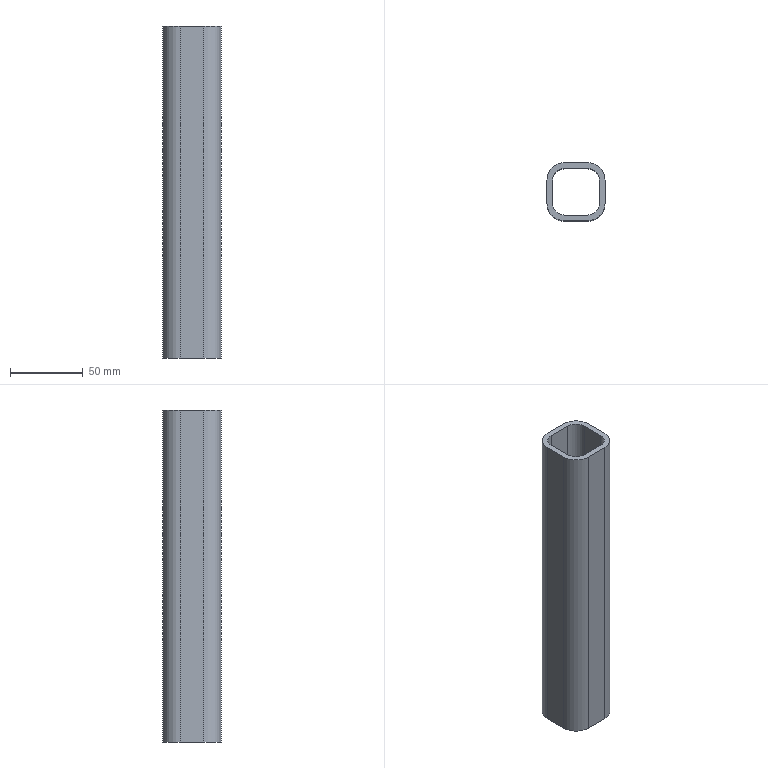Part | SolidWorks | features BaseBody 1 | 1 solid | 18 faces | box 40 x 40 x 228 mm | volume 115671 mm3 | plane 10 | cylinder 8 | commonest cylinder face diameters 16 x4 24 x4
STEP:
#1=CARTESIAN_POINT('',(8.,-20.,0.));
#2=VERTEX_POINT('',#1);
#3=CARTESIAN_POINT('',(20.,-8.,0.));
#4=VERTEX_POINT('',#3);
#5=CARTESIAN_POINT('',(8.,-8.,0.));
#6=DIRECTION('',(0.,0.,1.));
#7=DIRECTION('',(1.,0.,0.));
#8=AXIS2_PLACEMENT_3D('',#5,#6,#7);
#9=CIRCLE('',#8,12.);
#10=EDGE_CURVE('',#2,#4,#9,.T.);
#11=ORIENTED_EDGE('',*,*,#10,.T.);
#12=CARTESIAN_POINT('',(20.,-8.,228.));
#13=VERTEX_POINT('',#12);
#14=CARTESIAN_POINT('',(20.,-8.,0.));
#15=DIRECTION('',(0.,0.,1.));
#16=VECTOR('',#15,1000.);
#17=LINE('',#14,#16);
#18=EDGE_CURVE('',#4,#13,#17,.T.);
#19=ORIENTED_EDGE('',*,*,#18,.T.);
#20=CARTESIAN_POINT('',(8.,-20.,228.));
#21=VERTEX_POINT('',#20);
#22=CARTESIAN_POINT('',(8.,-8.,228.));
#23=DIRECTION('',(0.,0.,-1.));
#24=DIRECTION('',(1.,0.,0.));
#25=AXIS2_PLACEMENT_3D('',#22,#23,#24);
#26=CIRCLE('',#25,12.);
#27=EDGE_CURVE('',#13,#21,#26,.T.);
#28=ORIENTED_EDGE('',*,*,#27,.T.);
#29=CARTESIAN_POINT('',(8.,-20.,0.));
#30=DIRECTION('',(0.,0.,-1.));
#31=VECTOR('',#30,1000.);
#32=LINE('',#29,#31);
#33=EDGE_CURVE('',#21,#2,#32,.T.);
#34=ORIENTED_EDGE('',*,*,#33,.T.);
#35=EDGE_LOOP('',(#11,#19,#28,#34));
#36=FACE_OUTER_BOUND('',#35,.T.);
#37=CARTESIAN_POINT('',(8.,-8.,0.));
#38=DIRECTION('',(0.,0.,1.));
#39=DIRECTION('',(1.,0.,0.));
#40=AXIS2_PLACEMENT_3D('',#37,#38,#39);
#41=CYLINDRICAL_SURFACE('',#40,12.);
#42=ADVANCED_FACE('',(#36),#41,.T.);
#43=CARTESIAN_POINT('',(20.,8.,0.));
#44=VERTEX_POINT('',#43);
#45=CARTESIAN_POINT('',(20.,8.,0.));
#46=DIRECTION('',(0.,1.,0.));
#47=VECTOR('',#46,1000.);
#48=LINE('',#45,#47);
#49=EDGE_CURVE('',#4,#44,#48,.T.);
#50=ORIENTED_EDGE('',*,*,#49,.T.);
#51=CARTESIAN_POINT('',(20.,8.,228.));
#52=VERTEX_POINT('',#51);
#53=CARTESIAN_POINT('',(20.,8.,0.));
#54=DIRECTION('',(0.,0.,1.));
#55=VECTOR('',#54,1000.);
#56=LINE('',#53,#55);
#57=EDGE_CURVE('',#44,#52,#56,.T.);
#58=ORIENTED_EDGE('',*,*,#57,.T.);
#59=CARTESIAN_POINT('',(20.,8.,228.));
#60=DIRECTION('',(0.,-1.,0.));
#61=VECTOR('',#60,1000.);
#62=LINE('',#59,#61);
#63=EDGE_CURVE('',#52,#13,#62,.T.);
#64=ORIENTED_EDGE('',*,*,#63,.T.);
#65=ORIENTED_EDGE('',*,*,#18,.F.);
#66=EDGE_LOOP('',(#50,#58,#64,#65));
#67=FACE_OUTER_BOUND('',#66,.T.);
#68=CARTESIAN_POINT('',(20.,8.,0.));
#69=DIRECTION('',(1.,0.,0.));
#70=DIRECTION('',(0.,1.,0.));
#71=AXIS2_PLACEMENT_3D('',#68,#69,#70);
#72=PLANE('',#71);
#73=ADVANCED_FACE('',(#67),#72,.T.);
#74=CARTESIAN_POINT('',(-16.,8.,0.));
#75=VERTEX_POINT('',#74);
#76=CARTESIAN_POINT('',(-8.,16.,0.));
#77=VERTEX_POINT('',#76);
#78=CARTESIAN_POINT('',(-8.,8.,0.));
#79=DIRECTION('',(0.,0.,-1.));
#80=DIRECTION('',(1.,0.,0.));
#81=AXIS2_PLACEMENT_3D('',#78,#79,#80);
#82=CIRCLE('',#81,8.);
#83=EDGE_CURVE('',#75,#77,#82,.T.);
#84=ORIENTED_EDGE('',*,*,#83,.F.);
#85=CARTESIAN_POINT('',(-16.,-8.,0.));
#86=VERTEX_POINT('',#85);
#87=CARTESIAN_POINT('',(-16.,0.,0.));
#88=DIRECTION('',(0.,1.,0.));
#89=VECTOR('',#88,1000.);
#90=LINE('',#87,#89);
#91=EDGE_CURVE('',#86,#75,#90,.T.);
#92=ORIENTED_EDGE('',*,*,#91,.F.);
#93=CARTESIAN_POINT('',(-8.,-16.,0.));
#94=VERTEX_POINT('',#93);
#95=CARTESIAN_POINT('',(-8.,-8.,0.));
#96=DIRECTION('',(0.,0.,-1.));
#97=DIRECTION('',(1.,0.,0.));
#98=AXIS2_PLACEMENT_3D('',#95,#96,#97);
#99=CIRCLE('',#98,8.);
#100=EDGE_CURVE('',#94,#86,#99,.T.);
#101=ORIENTED_EDGE('',*,*,#100,.F.);
#102=CARTESIAN_POINT('',(8.,-16.,0.));
#103=VERTEX_POINT('',#102);
#104=CARTESIAN_POINT('',(0.,-16.,0.));
#105=DIRECTION('',(-1.,0.,0.));
#106=VECTOR('',#105,1000.);
#107=LINE('',#104,#106);
#108=EDGE_CURVE('',#103,#94,#107,.T.);
#109=ORIENTED_EDGE('',*,*,#108,.F.);
#110=CARTESIAN_POINT('',(16.,-8.,0.));
#111=VERTEX_POINT('',#110);
#112=CARTESIAN_POINT('',(8.,-8.,0.));
#113=DIRECTION('',(0.,0.,-1.));
#114=DIRECTION('',(1.,0.,0.));
#115=AXIS2_PLACEMENT_3D('',#112,#113,#114);
#116=CIRCLE('',#115,8.);
#117=EDGE_CURVE('',#111,#103,#116,.T.);
#118=ORIENTED_EDGE('',*,*,#117,.F.);
#119=CARTESIAN_POINT('',(16.,8.,0.));
#120=VERTEX_POINT('',#119);
#121=CARTESIAN_POINT('',(16.,0.,0.));
#122=DIRECTION('',(0.,-1.,0.));
#123=VECTOR('',#122,1000.);
#124=LINE('',#121,#123);
#125=EDGE_CURVE('',#120,#111,#124,.T.);
#126=ORIENTED_EDGE('',*,*,#125,.F.);
#127=CARTESIAN_POINT('',(8.,16.,0.));
#128=VERTEX_POINT('',#127);
#129=CARTESIAN_POINT('',(8.,8.,0.));
#130=DIRECTION('',(0.,0.,-1.));
#131=DIRECTION('',(1.,0.,0.));
#132=AXIS2_PLACEMENT_3D('',#129,#130,#131);
#133=CIRCLE('',#132,8.);
#134=EDGE_CURVE('',#128,#120,#133,.T.);
#135=ORIENTED_EDGE('',*,*,#134,.F.);
#136=CARTESIAN_POINT('',(0.,16.,0.));
#137=DIRECTION('',(1.,0.,0.));
#138=VECTOR('',#137,1000.);
#139=LINE('',#136,#138);
#140=EDGE_CURVE('',#77,#128,#139,.T.);
#141=ORIENTED_EDGE('',*,*,#140,.F.);
#142=EDGE_LOOP('',(#84,#92,#101,#109,#118,#126,#135,#141));
#143=FACE_BOUND('',#142,.T.);
#144=CARTESIAN_POINT('',(-8.,20.,0.));
#145=VERTEX_POINT('',#144);
#146=CARTESIAN_POINT('',(-20.,8.,0.));
#147=VERTEX_POINT('',#146);
#148=CARTESIAN_POINT('',(-8.,8.,0.));
#149=DIRECTION('',(0.,0.,1.));
#150=DIRECTION('',(1.,0.,0.));
#151=AXIS2_PLACEMENT_3D('',#148,#149,#150);
#152=CIRCLE('',#151,12.);
#153=EDGE_CURVE('',#145,#147,#152,.T.);
#154=ORIENTED_EDGE('',*,*,#153,.F.);
#155=CARTESIAN_POINT('',(8.,20.,0.));
#156=VERTEX_POINT('',#155);
#157=CARTESIAN_POINT('',(0.,20.,0.));
#158=DIRECTION('',(-1.,0.,0.));
#159=VECTOR('',#158,1000.);
#160=LINE('',#157,#159);
#161=EDGE_CURVE('',#156,#145,#160,.T.);
#162=ORIENTED_EDGE('',*,*,#161,.F.);
#163=CARTESIAN_POINT('',(8.,8.,0.));
#164=DIRECTION('',(0.,0.,1.));
#165=DIRECTION('',(1.,0.,0.));
#166=AXIS2_PLACEMENT_3D('',#163,#164,#165);
#167=CIRCLE('',#166,12.);
#168=EDGE_CURVE('',#44,#156,#167,.T.);
#169=ORIENTED_EDGE('',*,*,#168,.F.);
#170=ORIENTED_EDGE('',*,*,#49,.F.);
#171=ORIENTED_EDGE('',*,*,#10,.F.);
#172=CARTESIAN_POINT('',(-8.,-20.,0.));
#173=VERTEX_POINT('',#172);
#174=CARTESIAN_POINT('',(0.,-20.,0.));
#175=DIRECTION('',(1.,0.,0.));
#176=VECTOR('',#175,1000.);
#177=LINE('',#174,#176);
#178=EDGE_CURVE('',#173,#2,#177,.T.);
#179=ORIENTED_EDGE('',*,*,#178,.F.);
#180=CARTESIAN_POINT('',(-20.,-8.,0.));
#181=VERTEX_POINT('',#180);
#182=CARTESIAN_POINT('',(-8.,-8.,0.));
#183=DIRECTION('',(0.,0.,1.));
#184=DIRECTION('',(1.,0.,0.));
#185=AXIS2_PLACEMENT_3D('',#182,#183,#184);
#186=CIRCLE('',#185,12.);
#187=EDGE_CURVE('',#181,#173,#186,.T.);
#188=ORIENTED_EDGE('',*,*,#187,.F.);
#189=CARTESIAN_POINT('',(-20.,0.,0.));
#190=DIRECTION('',(0.,-1.,0.));
#191=VECTOR('',#190,1000.);
#192=LINE('',#189,#191);
#193=EDGE_CURVE('',#147,#181,#192,.T.);
#194=ORIENTED_EDGE('',*,*,#193,.F.);
#195=EDGE_LOOP('',(#154,#162,#169,#170,#171,#179,#188,#194));
#196=FACE_OUTER_BOUND('',#195,.T.);
#197=CARTESIAN_POINT('',(0.,0.,0.));
#198=DIRECTION('',(0.,0.,1.));
#199=DIRECTION('',(1.,0.,0.));
#200=AXIS2_PLACEMENT_3D('',#197,#198,#199);
#201=PLANE('',#200);
#202=ADVANCED_FACE('',(#143,#196),#201,.F.);
#203=ORIENTED_EDGE('',*,*,#178,.T.);
#204=ORIENTED_EDGE('',*,*,#33,.F.);
#205=CARTESIAN_POINT('',(-8.,-20.,228.));
#206=VERTEX_POINT('',#205);
#207=CARTESIAN_POINT('',(8.,-20.,228.));
#208=DIRECTION('',(-1.,0.,0.));
#209=VECTOR('',#208,1000.);
#210=LINE('',#207,#209);
#211=EDGE_CURVE('',#21,#206,#210,.T.);
#212=ORIENTED_EDGE('',*,*,#211,.T.);
#213=CARTESIAN_POINT('',(-8.,-20.,0.));
#214=DIRECTION('',(0.,0.,-1.));
#215=VECTOR('',#214,1000.);
#216=LINE('',#213,#215);
#217=EDGE_CURVE('',#206,#173,#216,.T.);
#218=ORIENTED_EDGE('',*,*,#217,.T.);
#219=EDGE_LOOP('',(#203,#204,#212,#218));
#220=FACE_OUTER_BOUND('',#219,.T.);
#221=CARTESIAN_POINT('',(8.,-20.,0.));
#222=DIRECTION('',(0.,-1.,0.));
#223=DIRECTION('',(1.,0.,0.));
#224=AXIS2_PLACEMENT_3D('',#221,#222,#223);
#225=PLANE('',#224);
#226=ADVANCED_FACE('',(#220),#225,.T.);
#227=CARTESIAN_POINT('',(-16.,-8.,228.));
#228=VERTEX_POINT('',#227);
#229=CARTESIAN_POINT('',(-16.,8.,228.));
#230=VERTEX_POINT('',#229);
#231=CARTESIAN_POINT('',(-16.,0.,228.));
#232=DIRECTION('',(0.,1.,0.));
#233=VECTOR('',#232,1000.);
#234=LINE('',#231,#233);
#235=EDGE_CURVE('',#228,#230,#234,.T.);
#236=ORIENTED_EDGE('',*,*,#235,.T.);
#237=CARTESIAN_POINT('',(-8.,16.,228.));
#238=VERTEX_POINT('',#237);
#239=CARTESIAN_POINT('',(-8.,8.,228.));
#240=DIRECTION('',(0.,0.,-1.));
#241=DIRECTION('',(1.,0.,0.));
#242=AXIS2_PLACEMENT_3D('',#239,#240,#241);
#243=CIRCLE('',#242,8.);
#244=EDGE_CURVE('',#230,#238,#243,.T.);
#245=ORIENTED_EDGE('',*,*,#244,.T.);
#246=CARTESIAN_POINT('',(8.,16.,228.));
#247=VERTEX_POINT('',#246);
#248=CARTESIAN_POINT('',(0.,16.,228.));
#249=DIRECTION('',(1.,0.,0.));
#250=VECTOR('',#249,1000.);
#251=LINE('',#248,#250);
#252=EDGE_CURVE('',#238,#247,#251,.T.);
#253=ORIENTED_EDGE('',*,*,#252,.T.);
#254=CARTESIAN_POINT('',(16.,8.,228.));
#255=VERTEX_POINT('',#254);
#256=CARTESIAN_POINT('',(8.,8.,228.));
#257=DIRECTION('',(0.,0.,-1.));
#258=DIRECTION('',(1.,0.,0.));
#259=AXIS2_PLACEMENT_3D('',#256,#257,#258);
#260=CIRCLE('',#259,8.);
#261=EDGE_CURVE('',#247,#255,#260,.T.);
#262=ORIENTED_EDGE('',*,*,#261,.T.);
#263=CARTESIAN_POINT('',(16.,-8.,228.));
#264=VERTEX_POINT('',#263);
#265=CARTESIAN_POINT('',(16.,0.,228.));
#266=DIRECTION('',(0.,-1.,0.));
#267=VECTOR('',#266,1000.);
#268=LINE('',#265,#267);
#269=EDGE_CURVE('',#255,#264,#268,.T.);
#270=ORIENTED_EDGE('',*,*,#269,.T.);
#271=CARTESIAN_POINT('',(8.,-16.,228.));
#272=VERTEX_POINT('',#271);
#273=CARTESIAN_POINT('',(8.,-8.,228.));
#274=DIRECTION('',(0.,0.,-1.));
#275=DIRECTION('',(1.,0.,0.));
#276=AXIS2_PLACEMENT_3D('',#273,#274,#275);
#277=CIRCLE('',#276,8.);
#278=EDGE_CURVE('',#264,#272,#277,.T.);
#279=ORIENTED_EDGE('',*,*,#278,.T.);
#280=CARTESIAN_POINT('',(-8.,-16.,228.));
#281=VERTEX_POINT('',#280);
#282=CARTESIAN_POINT('',(0.,-16.,228.));
#283=DIRECTION('',(-1.,0.,0.));
#284=VECTOR('',#283,1000.);
#285=LINE('',#282,#284);
#286=EDGE_CURVE('',#272,#281,#285,.T.);
#287=ORIENTED_EDGE('',*,*,#286,.T.);
#288=CARTESIAN_POINT('',(-8.,-8.,228.));
#289=DIRECTION('',(0.,0.,-1.));
#290=DIRECTION('',(1.,0.,0.));
#291=AXIS2_PLACEMENT_3D('',#288,#289,#290);
#292=CIRCLE('',#291,8.);
#293=EDGE_CURVE('',#281,#228,#292,.T.);
#294=ORIENTED_EDGE('',*,*,#293,.T.);
#295=EDGE_LOOP('',(#236,#245,#253,#262,#270,#279,#287,#294));
#296=FACE_BOUND('',#295,.T.);
#297=CARTESIAN_POINT('',(8.,20.,228.));
#298=VERTEX_POINT('',#297);
#299=CARTESIAN_POINT('',(-8.,20.,228.));
#300=VERTEX_POINT('',#299);
#301=CARTESIAN_POINT('',(0.,20.,228.));
#302=DIRECTION('',(-1.,0.,0.));
#303=VECTOR('',#302,1000.);
#304=LINE('',#301,#303);
#305=EDGE_CURVE('',#298,#300,#304,.T.);
#306=ORIENTED_EDGE('',*,*,#305,.T.);
#307=CARTESIAN_POINT('',(-20.,8.,228.));
#308=VERTEX_POINT('',#307);
#309=CARTESIAN_POINT('',(-8.,8.,228.));
#310=DIRECTION('',(0.,0.,1.));
#311=DIRECTION('',(1.,0.,0.));
#312=AXIS2_PLACEMENT_3D('',#309,#310,#311);
#313=CIRCLE('',#312,12.);
#314=EDGE_CURVE('',#300,#308,#313,.T.);
#315=ORIENTED_EDGE('',*,*,#314,.T.);
#316=CARTESIAN_POINT('',(-20.,-8.,228.));
#317=VERTEX_POINT('',#316);
#318=CARTESIAN_POINT('',(-20.,0.,228.));
#319=DIRECTION('',(0.,-1.,0.));
#320=VECTOR('',#319,1000.);
#321=LINE('',#318,#320);
#322=EDGE_CURVE('',#308,#317,#321,.T.);
#323=ORIENTED_EDGE('',*,*,#322,.T.);
#324=CARTESIAN_POINT('',(-8.,-8.,228.));
#325=DIRECTION('',(0.,0.,1.));
#326=DIRECTION('',(1.,0.,0.));
#327=AXIS2_PLACEMENT_3D('',#324,#325,#326);
#328=CIRCLE('',#327,12.);
#329=EDGE_CURVE('',#317,#206,#328,.T.);
#330=ORIENTED_EDGE('',*,*,#329,.T.);
#331=ORIENTED_EDGE('',*,*,#211,.F.);
#332=ORIENTED_EDGE('',*,*,#27,.F.);
#333=ORIENTED_EDGE('',*,*,#63,.F.);
#334=CARTESIAN_POINT('',(8.,8.,228.));
#335=DIRECTION('',(0.,0.,1.));
#336=DIRECTION('',(1.,0.,0.));
#337=AXIS2_PLACEMENT_3D('',#334,#335,#336);
#338=CIRCLE('',#337,12.);
#339=EDGE_CURVE('',#52,#298,#338,.T.);
#340=ORIENTED_EDGE('',*,*,#339,.T.);
#341=EDGE_LOOP('',(#306,#315,#323,#330,#331,#332,#333,#340));
#342=FACE_OUTER_BOUND('',#341,.T.);
#343=CARTESIAN_POINT('',(0.,0.,228.));
#344=DIRECTION('',(0.,0.,1.));
#345=DIRECTION('',(1.,0.,0.));
#346=AXIS2_PLACEMENT_3D('',#343,#344,#345);
#347=PLANE('',#346);
#348=ADVANCED_FACE('',(#296,#342),#347,.T.);
#349=ORIENTED_EDGE('',*,*,#168,.T.);
#350=CARTESIAN_POINT('',(8.,20.,0.));
#351=DIRECTION('',(0.,0.,1.));
#352=VECTOR('',#351,1000.);
#353=LINE('',#350,#352);
#354=EDGE_CURVE('',#156,#298,#353,.T.);
#355=ORIENTED_EDGE('',*,*,#354,.T.);
#356=ORIENTED_EDGE('',*,*,#339,.F.);
#357=ORIENTED_EDGE('',*,*,#57,.F.);
#358=EDGE_LOOP('',(#349,#355,#356,#357));
#359=FACE_OUTER_BOUND('',#358,.T.);
#360=CARTESIAN_POINT('',(8.,8.,0.));
#361=DIRECTION('',(0.,0.,1.));
#362=DIRECTION('',(1.,0.,0.));
#363=AXIS2_PLACEMENT_3D('',#360,#361,#362);
#364=CYLINDRICAL_SURFACE('',#363,12.);
#365=ADVANCED_FACE('',(#359),#364,.T.);
#366=CARTESIAN_POINT('',(-8.,16.,0.));
#367=DIRECTION('',(0.,0.,1.));
#368=VECTOR('',#367,1000.);
#369=LINE('',#366,#368);
#370=EDGE_CURVE('',#77,#238,#369,.T.);
#371=ORIENTED_EDGE('',*,*,#370,.F.);
#372=ORIENTED_EDGE('',*,*,#140,.T.);
#373=CARTESIAN_POINT('',(8.,16.,0.));
#374=DIRECTION('',(0.,0.,-1.));
#375=VECTOR('',#374,1000.);
#376=LINE('',#373,#375);
#377=EDGE_CURVE('',#247,#128,#376,.T.);
#378=ORIENTED_EDGE('',*,*,#377,.F.);
#379=ORIENTED_EDGE('',*,*,#252,.F.);
#380=EDGE_LOOP('',(#371,#372,#378,#379));
#381=FACE_OUTER_BOUND('',#380,.T.);
#382=CARTESIAN_POINT('',(-8.,16.,0.));
#383=DIRECTION('',(0.,1.,0.));
#384=DIRECTION('',(-1.,0.,0.));
#385=AXIS2_PLACEMENT_3D('',#382,#383,#384);
#386=PLANE('',#385);
#387=ADVANCED_FACE('',(#381),#386,.F.);
#388=CARTESIAN_POINT('',(-16.,8.,0.));
#389=DIRECTION('',(0.,0.,1.));
#390=VECTOR('',#389,1000.);
#391=LINE('',#388,#390);
#392=EDGE_CURVE('',#75,#230,#391,.T.);
#393=ORIENTED_EDGE('',*,*,#392,.F.);
#394=ORIENTED_EDGE('',*,*,#83,.T.);
#395=ORIENTED_EDGE('',*,*,#370,.T.);
#396=ORIENTED_EDGE('',*,*,#244,.F.);
#397=EDGE_LOOP('',(#393,#394,#395,#396));
#398=FACE_OUTER_BOUND('',#397,.T.);
#399=CARTESIAN_POINT('',(-8.,8.,0.));
#400=DIRECTION('',(0.,0.,1.));
#401=DIRECTION('',(1.,0.,0.));
#402=AXIS2_PLACEMENT_3D('',#399,#400,#401);
#403=CYLINDRICAL_SURFACE('',#402,8.);
#404=ADVANCED_FACE('',(#398),#403,.F.);
#405=CARTESIAN_POINT('',(-16.,-8.,0.));
#406=DIRECTION('',(0.,0.,1.));
#407=VECTOR('',#406,1000.);
#408=LINE('',#405,#407);
#409=EDGE_CURVE('',#86,#228,#408,.T.);
#410=ORIENTED_EDGE('',*,*,#409,.F.);
#411=ORIENTED_EDGE('',*,*,#91,.T.);
#412=ORIENTED_EDGE('',*,*,#392,.T.);
#413=ORIENTED_EDGE('',*,*,#235,.F.);
#414=EDGE_LOOP('',(#410,#411,#412,#413));
#415=FACE_OUTER_BOUND('',#414,.T.);
#416=CARTESIAN_POINT('',(-16.,-8.,0.));
#417=DIRECTION('',(-1.,0.,0.));
#418=DIRECTION('',(0.,-1.,0.));
#419=AXIS2_PLACEMENT_3D('',#416,#417,#418);
#420=PLANE('',#419);
#421=ADVANCED_FACE('',(#415),#420,.F.);
#422=CARTESIAN_POINT('',(-8.,-16.,0.));
#423=DIRECTION('',(0.,0.,1.));
#424=VECTOR('',#423,1000.);
#425=LINE('',#422,#424);
#426=EDGE_CURVE('',#94,#281,#425,.T.);
#427=ORIENTED_EDGE('',*,*,#426,.F.);
#428=ORIENTED_EDGE('',*,*,#100,.T.);
#429=ORIENTED_EDGE('',*,*,#409,.T.);
#430=ORIENTED_EDGE('',*,*,#293,.F.);
#431=EDGE_LOOP('',(#427,#428,#429,#430));
#432=FACE_OUTER_BOUND('',#431,.T.);
#433=CARTESIAN_POINT('',(-8.,-8.,0.));
#434=DIRECTION('',(0.,0.,1.));
#435=DIRECTION('',(1.,0.,0.));
#436=AXIS2_PLACEMENT_3D('',#433,#434,#435);
#437=CYLINDRICAL_SURFACE('',#436,8.);
#438=ADVANCED_FACE('',(#432),#437,.F.);
#439=CARTESIAN_POINT('',(8.,-16.,0.));
#440=DIRECTION('',(0.,0.,1.));
#441=VECTOR('',#440,1000.);
#442=LINE('',#439,#441);
#443=EDGE_CURVE('',#103,#272,#442,.T.);
#444=ORIENTED_EDGE('',*,*,#443,.F.);
#445=ORIENTED_EDGE('',*,*,#108,.T.);
#446=ORIENTED_EDGE('',*,*,#426,.T.);
#447=ORIENTED_EDGE('',*,*,#286,.F.);
#448=EDGE_LOOP('',(#444,#445,#446,#447));
#449=FACE_OUTER_BOUND('',#448,.T.);
#450=CARTESIAN_POINT('',(8.,-16.,0.));
#451=DIRECTION('',(0.,-1.,0.));
#452=DIRECTION('',(1.,0.,0.));
#453=AXIS2_PLACEMENT_3D('',#450,#451,#452);
#454=PLANE('',#453);
#455=ADVANCED_FACE('',(#449),#454,.F.);
#456=CARTESIAN_POINT('',(16.,-8.,0.));
#457=DIRECTION('',(0.,0.,1.));
#458=VECTOR('',#457,1000.);
#459=LINE('',#456,#458);
#460=EDGE_CURVE('',#111,#264,#459,.T.);
#461=ORIENTED_EDGE('',*,*,#460,.F.);
#462=ORIENTED_EDGE('',*,*,#117,.T.);
#463=ORIENTED_EDGE('',*,*,#443,.T.);
#464=ORIENTED_EDGE('',*,*,#278,.F.);
#465=EDGE_LOOP('',(#461,#462,#463,#464));
#466=FACE_OUTER_BOUND('',#465,.T.);
#467=CARTESIAN_POINT('',(8.,-8.,0.));
#468=DIRECTION('',(0.,0.,1.));
#469=DIRECTION('',(1.,0.,0.));
#470=AXIS2_PLACEMENT_3D('',#467,#468,#469);
#471=CYLINDRICAL_SURFACE('',#470,8.);
#472=ADVANCED_FACE('',(#466),#471,.F.);
#473=CARTESIAN_POINT('',(16.,8.,0.));
#474=DIRECTION('',(0.,0.,1.));
#475=VECTOR('',#474,1000.);
#476=LINE('',#473,#475);
#477=EDGE_CURVE('',#120,#255,#476,.T.);
#478=ORIENTED_EDGE('',*,*,#477,.F.);
#479=ORIENTED_EDGE('',*,*,#125,.T.);
#480=ORIENTED_EDGE('',*,*,#460,.T.);
#481=ORIENTED_EDGE('',*,*,#269,.F.);
#482=EDGE_LOOP('',(#478,#479,#480,#481));
#483=FACE_OUTER_BOUND('',#482,.T.);
#484=CARTESIAN_POINT('',(16.,8.,0.));
#485=DIRECTION('',(1.,0.,0.));
#486=DIRECTION('',(0.,0.,-1.));
#487=AXIS2_PLACEMENT_3D('',#484,#485,#486);
#488=PLANE('',#487);
#489=ADVANCED_FACE('',(#483),#488,.F.);
#490=ORIENTED_EDGE('',*,*,#377,.T.);
#491=ORIENTED_EDGE('',*,*,#134,.T.);
#492=ORIENTED_EDGE('',*,*,#477,.T.);
#493=ORIENTED_EDGE('',*,*,#261,.F.);
#494=EDGE_LOOP('',(#490,#491,#492,#493));
#495=FACE_OUTER_BOUND('',#494,.T.);
#496=CARTESIAN_POINT('',(8.,8.,0.));
#497=DIRECTION('',(0.,0.,1.));
#498=DIRECTION('',(1.,0.,0.));
#499=AXIS2_PLACEMENT_3D('',#496,#497,#498);
#500=CYLINDRICAL_SURFACE('',#499,8.);
#501=ADVANCED_FACE('',(#495),#500,.F.);
#502=ORIENTED_EDGE('',*,*,#193,.T.);
#503=CARTESIAN_POINT('',(-20.,-8.,0.));
#504=DIRECTION('',(0.,0.,1.));
#505=VECTOR('',#504,1000.);
#506=LINE('',#503,#505);
#507=EDGE_CURVE('',#181,#317,#506,.T.);
#508=ORIENTED_EDGE('',*,*,#507,.T.);
#509=ORIENTED_EDGE('',*,*,#322,.F.);
#510=CARTESIAN_POINT('',(-20.,8.,0.));
#511=DIRECTION('',(0.,0.,-1.));
#512=VECTOR('',#511,1000.);
#513=LINE('',#510,#512);
#514=EDGE_CURVE('',#308,#147,#513,.T.);
#515=ORIENTED_EDGE('',*,*,#514,.T.);
#516=EDGE_LOOP('',(#502,#508,#509,#515));
#517=FACE_OUTER_BOUND('',#516,.T.);
#518=CARTESIAN_POINT('',(-20.,-8.,0.));
#519=DIRECTION('',(-1.,0.,0.));
#520=DIRECTION('',(0.,-1.,0.));
#521=AXIS2_PLACEMENT_3D('',#518,#519,#520);
#522=PLANE('',#521);
#523=ADVANCED_FACE('',(#517),#522,.T.);
#524=ORIENTED_EDGE('',*,*,#153,.T.);
#525=ORIENTED_EDGE('',*,*,#514,.F.);
#526=ORIENTED_EDGE('',*,*,#314,.F.);
#527=CARTESIAN_POINT('',(-8.,20.,0.));
#528=DIRECTION('',(0.,0.,-1.));
#529=VECTOR('',#528,1000.);
#530=LINE('',#527,#529);
#531=EDGE_CURVE('',#300,#145,#530,.T.);
#532=ORIENTED_EDGE('',*,*,#531,.T.);
#533=EDGE_LOOP('',(#524,#525,#526,#532));
#534=FACE_OUTER_BOUND('',#533,.T.);
#535=CARTESIAN_POINT('',(-8.,8.,0.));
#536=DIRECTION('',(0.,0.,1.));
#537=DIRECTION('',(1.,0.,0.));
#538=AXIS2_PLACEMENT_3D('',#535,#536,#537);
#539=CYLINDRICAL_SURFACE('',#538,12.);
#540=ADVANCED_FACE('',(#534),#539,.T.);
#541=ORIENTED_EDGE('',*,*,#161,.T.);
#542=ORIENTED_EDGE('',*,*,#531,.F.);
#543=ORIENTED_EDGE('',*,*,#305,.F.);
#544=ORIENTED_EDGE('',*,*,#354,.F.);
#545=EDGE_LOOP('',(#541,#542,#543,#544));
#546=FACE_OUTER_BOUND('',#545,.T.);
#547=CARTESIAN_POINT('',(-8.,20.,0.));
#548=DIRECTION('',(0.,1.,0.));
#549=DIRECTION('',(0.,0.,1.));
#550=AXIS2_PLACEMENT_3D('',#547,#548,#549);
#551=PLANE('',#550);
#552=ADVANCED_FACE('',(#546),#551,.T.);
#553=ORIENTED_EDGE('',*,*,#187,.T.);
#554=ORIENTED_EDGE('',*,*,#217,.F.);
#555=ORIENTED_EDGE('',*,*,#329,.F.);
#556=ORIENTED_EDGE('',*,*,#507,.F.);
#557=EDGE_LOOP('',(#553,#554,#555,#556));
#558=FACE_OUTER_BOUND('',#557,.T.);
#559=CARTESIAN_POINT('',(-8.,-8.,0.));
#560=DIRECTION('',(0.,0.,1.));
#561=DIRECTION('',(1.,0.,0.));
#562=AXIS2_PLACEMENT_3D('',#559,#560,#561);
#563=CYLINDRICAL_SURFACE('',#562,12.);
#564=ADVANCED_FACE('',(#558),#563,.T.);
#565=CLOSED_SHELL('',(#42,#73,#202,#226,#348,#365,#387,#404,#421,#438,#455,#472,#489,#501,#523,#540,#552,#564));
#566=MANIFOLD_SOLID_BREP('',#565);
#567=CARTESIAN_POINT('',(0.,0.,0.));
#568=DIRECTION('',(0.,0.,1.));
#569=DIRECTION('',(1.,0.,0.));
#570=AXIS2_PLACEMENT_3D('',#567,#568,#569);
#571=(LENGTH_UNIT()NAMED_UNIT(*)SI_UNIT(.MILLI.,.METRE.));
#572=UNCERTAINTY_MEASURE_WITH_UNIT(LENGTH_MEASURE(0.00001),#571,'','');
#573=(NAMED_UNIT(*)PLANE_ANGLE_UNIT()SI_UNIT($,.RADIAN.));
#574=(NAMED_UNIT(*)SI_UNIT($,.STERADIAN.)SOLID_ANGLE_UNIT());
#575=(GEOMETRIC_REPRESENTATION_CONTEXT(3)GLOBAL_UNCERTAINTY_ASSIGNED_CONTEXT((#572))GLOBAL_UNIT_ASSIGNED_CONTEXT((#571,#573,#574))REPRESENTATION_CONTEXT('',''));
#576=ADVANCED_BREP_SHAPE_REPRESENTATION('',(#566,#570),#575);